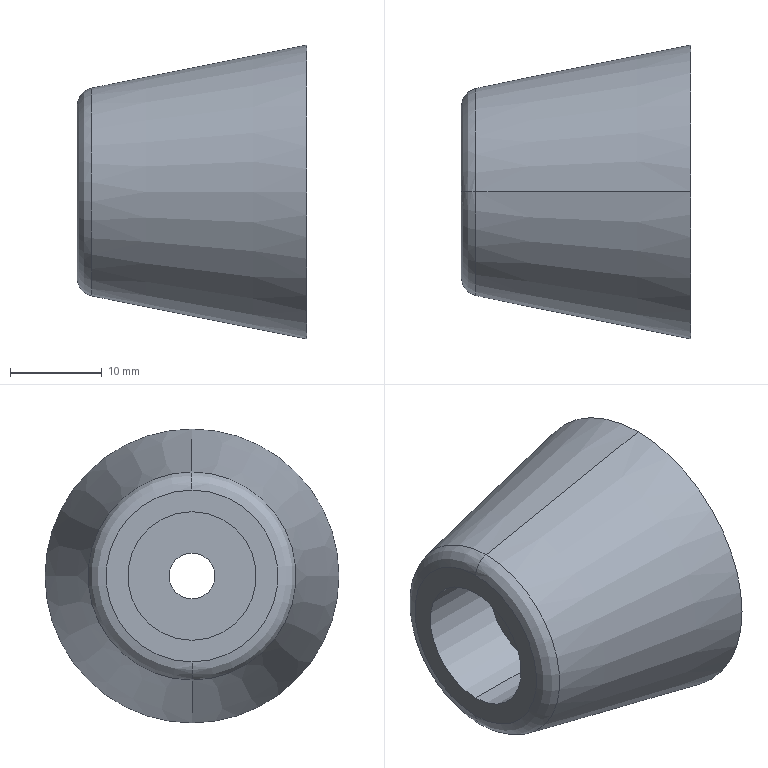Part | STEP file | NHY11-32 | 1 solid | 11 faces | box 25 x 32 x 32 mm | volume 12742 mm3 | cylinder 4 | plane 3 | cone 2 | torus 2 | commonest cylinder face diameters 5 x2 14 x2
STEP:
#1=CARTESIAN_POINT('',(1.608,0.000000013,11.322));
#2=VERTEX_POINT('',#1);
#3=CARTESIAN_POINT('',(1.608,-0.000000013,-11.322));
#4=VERTEX_POINT('',#3);
#5=CARTESIAN_POINT('',(1.608,0.,0.));
#6=DIRECTION('',(1.,0.,0.));
#7=DIRECTION('',(0.,0.,-1.));
#8=AXIS2_PLACEMENT_3D('',#5,#6,#7);
#9=CIRCLE('',#8,11.322);
#10=EDGE_CURVE('',#2,#4,#9,.T.);
#11=ORIENTED_EDGE('',*,*,#10,.T.);
#12=CARTESIAN_POINT('',(25.,-0.000000012,-16.));
#13=VERTEX_POINT('',#12);
#14=CARTESIAN_POINT('',(25.,-0.000000012,-16.));
#15=DIRECTION('',(0.9806,0.,-0.1961));
#16=VECTOR('',#15,1000.);
#17=LINE('',#14,#16);
#18=EDGE_CURVE('',#4,#13,#17,.T.);
#19=ORIENTED_EDGE('',*,*,#18,.T.);
#20=CARTESIAN_POINT('',(25.,0.000000012,16.));
#21=VERTEX_POINT('',#20);
#22=CARTESIAN_POINT('',(25.,0.,0.));
#23=DIRECTION('',(1.,0.,0.));
#24=DIRECTION('',(0.,0.,1.));
#25=AXIS2_PLACEMENT_3D('',#22,#23,#24);
#26=CIRCLE('',#25,16.);
#27=EDGE_CURVE('',#21,#13,#26,.T.);
#28=ORIENTED_EDGE('',*,*,#27,.F.);
#29=CARTESIAN_POINT('',(25.,0.000000012,16.));
#30=DIRECTION('',(0.9806,0.,0.1961));
#31=VECTOR('',#30,1000.);
#32=LINE('',#29,#31);
#33=EDGE_CURVE('',#2,#21,#32,.T.);
#34=ORIENTED_EDGE('',*,*,#33,.F.);
#35=EDGE_LOOP('',(#11,#19,#28,#34));
#36=FACE_OUTER_BOUND('',#35,.T.);
#37=CARTESIAN_POINT('',(25.,0.,0.));
#38=DIRECTION('',(1.,0.,0.));
#39=DIRECTION('',(0.,0.000000001,1.));
#40=AXIS2_PLACEMENT_3D('',#37,#38,#39);
#41=CONICAL_SURFACE('',#40,16.,0.1974);
#42=ADVANCED_FACE('',(#36),#41,.T.);
#43=CARTESIAN_POINT('',(9.,0.,-2.5));
#44=VERTEX_POINT('',#43);
#45=CARTESIAN_POINT('',(9.,-0.000000355,2.5));
#46=VERTEX_POINT('',#45);
#47=CARTESIAN_POINT('',(9.,0.,0.));
#48=DIRECTION('',(1.,0.,0.));
#49=DIRECTION('',(0.,-0.000000142,1.));
#50=AXIS2_PLACEMENT_3D('',#47,#48,#49);
#51=CIRCLE('',#50,2.5);
#52=EDGE_CURVE('',#44,#46,#51,.T.);
#53=ORIENTED_EDGE('',*,*,#52,.F.);
#54=CARTESIAN_POINT('',(25.,0.,-2.5));
#55=VERTEX_POINT('',#54);
#56=CARTESIAN_POINT('',(25.,0.,-2.5));
#57=DIRECTION('',(1.,0.,0.));
#58=VECTOR('',#57,1000.);
#59=LINE('',#56,#58);
#60=EDGE_CURVE('',#44,#55,#59,.T.);
#61=ORIENTED_EDGE('',*,*,#60,.T.);
#62=CARTESIAN_POINT('',(25.,0.,2.5));
#63=VERTEX_POINT('',#62);
#64=CARTESIAN_POINT('',(25.,0.,0.));
#65=DIRECTION('',(1.,0.,0.));
#66=DIRECTION('',(0.,0.,-1.));
#67=AXIS2_PLACEMENT_3D('',#64,#65,#66);
#68=CIRCLE('',#67,2.5);
#69=EDGE_CURVE('',#55,#63,#68,.T.);
#70=ORIENTED_EDGE('',*,*,#69,.T.);
#71=CARTESIAN_POINT('',(25.,0.,2.5));
#72=DIRECTION('',(1.,0.,0.));
#73=VECTOR('',#72,1000.);
#74=LINE('',#71,#73);
#75=EDGE_CURVE('',#46,#63,#74,.T.);
#76=ORIENTED_EDGE('',*,*,#75,.F.);
#77=EDGE_LOOP('',(#53,#61,#70,#76));
#78=FACE_OUTER_BOUND('',#77,.T.);
#79=CARTESIAN_POINT('',(25.,0.,0.));
#80=DIRECTION('',(1.,0.,0.));
#81=DIRECTION('',(0.,0.,1.));
#82=AXIS2_PLACEMENT_3D('',#79,#80,#81);
#83=CYLINDRICAL_SURFACE('',#82,2.5);
#84=ADVANCED_FACE('',(#78),#83,.F.);
#85=CARTESIAN_POINT('',(0.,0.,-7.));
#86=VERTEX_POINT('',#85);
#87=CARTESIAN_POINT('',(0.,0.,7.));
#88=VERTEX_POINT('',#87);
#89=CARTESIAN_POINT('',(0.,0.,0.));
#90=DIRECTION('',(1.,0.,0.));
#91=DIRECTION('',(0.,0.,1.));
#92=AXIS2_PLACEMENT_3D('',#89,#90,#91);
#93=CIRCLE('',#92,7.);
#94=EDGE_CURVE('',#86,#88,#93,.T.);
#95=ORIENTED_EDGE('',*,*,#94,.F.);
#96=CARTESIAN_POINT('',(9.,0.,-7.));
#97=VERTEX_POINT('',#96);
#98=CARTESIAN_POINT('',(25.,0.,-7.));
#99=DIRECTION('',(1.,0.,0.));
#100=VECTOR('',#99,1000.);
#101=LINE('',#98,#100);
#102=EDGE_CURVE('',#86,#97,#101,.T.);
#103=ORIENTED_EDGE('',*,*,#102,.T.);
#104=CARTESIAN_POINT('',(9.,0.,7.));
#105=VERTEX_POINT('',#104);
#106=CARTESIAN_POINT('',(9.,0.,0.));
#107=DIRECTION('',(1.,0.,0.));
#108=DIRECTION('',(0.,0.,-1.));
#109=AXIS2_PLACEMENT_3D('',#106,#107,#108);
#110=CIRCLE('',#109,7.);
#111=EDGE_CURVE('',#97,#105,#110,.T.);
#112=ORIENTED_EDGE('',*,*,#111,.T.);
#113=CARTESIAN_POINT('',(25.,0.,7.));
#114=DIRECTION('',(1.,0.,0.));
#115=VECTOR('',#114,1000.);
#116=LINE('',#113,#115);
#117=EDGE_CURVE('',#88,#105,#116,.T.);
#118=ORIENTED_EDGE('',*,*,#117,.F.);
#119=EDGE_LOOP('',(#95,#103,#112,#118));
#120=FACE_OUTER_BOUND('',#119,.T.);
#121=CARTESIAN_POINT('',(25.,0.,0.));
#122=DIRECTION('',(1.,0.,0.));
#123=DIRECTION('',(0.,0.,1.));
#124=AXIS2_PLACEMENT_3D('',#121,#122,#123);
#125=CYLINDRICAL_SURFACE('',#124,7.);
#126=ADVANCED_FACE('',(#120),#125,.F.);
#127=CARTESIAN_POINT('',(0.,0.000000012,9.36));
#128=VERTEX_POINT('',#127);
#129=CARTESIAN_POINT('',(0.,-0.000000012,-9.36));
#130=VERTEX_POINT('',#129);
#131=CARTESIAN_POINT('',(0.,0.,0.));
#132=DIRECTION('',(1.,0.,0.));
#133=DIRECTION('',(0.,0.,-1.));
#134=AXIS2_PLACEMENT_3D('',#131,#132,#133);
#135=CIRCLE('',#134,9.36);
#136=EDGE_CURVE('',#128,#130,#135,.T.);
#137=ORIENTED_EDGE('',*,*,#136,.T.);
#138=CARTESIAN_POINT('',(2.,-0.000000011,-9.36));
#139=DIRECTION('',(0.,-1.,0.000000001));
#140=DIRECTION('',(0.,-0.000000001,-1.));
#141=AXIS2_PLACEMENT_3D('',#138,#139,#140);
#142=CIRCLE('',#141,2.);
#143=EDGE_CURVE('',#130,#4,#142,.T.);
#144=ORIENTED_EDGE('',*,*,#143,.T.);
#145=ORIENTED_EDGE('',*,*,#10,.F.);
#146=CARTESIAN_POINT('',(2.,0.000000011,9.36));
#147=DIRECTION('',(0.,1.,-0.000000001));
#148=DIRECTION('',(0.,0.000000001,1.));
#149=AXIS2_PLACEMENT_3D('',#146,#147,#148);
#150=CIRCLE('',#149,2.);
#151=EDGE_CURVE('',#128,#2,#150,.T.);
#152=ORIENTED_EDGE('',*,*,#151,.F.);
#153=EDGE_LOOP('',(#137,#144,#145,#152));
#154=FACE_OUTER_BOUND('',#153,.T.);
#155=CARTESIAN_POINT('',(2.,0.,0.));
#156=DIRECTION('',(1.,0.,0.));
#157=DIRECTION('',(0.,0.000000001,1.));
#158=AXIS2_PLACEMENT_3D('',#155,#156,#157);
#159=TOROIDAL_SURFACE('',#158,9.36,2.);
#160=ADVANCED_FACE('',(#154),#159,.T.);
#161=ORIENTED_EDGE('',*,*,#136,.F.);
#162=CARTESIAN_POINT('',(0.,0.,0.));
#163=DIRECTION('',(1.,0.,0.));
#164=DIRECTION('',(0.,0.,-1.));
#165=AXIS2_PLACEMENT_3D('',#162,#163,#164);
#166=CIRCLE('',#165,9.36);
#167=EDGE_CURVE('',#130,#128,#166,.T.);
#168=ORIENTED_EDGE('',*,*,#167,.F.);
#169=EDGE_LOOP('',(#161,#168));
#170=FACE_OUTER_BOUND('',#169,.T.);
#171=CARTESIAN_POINT('',(0.,0.,0.));
#172=DIRECTION('',(1.,0.,0.));
#173=DIRECTION('',(0.,0.,1.));
#174=AXIS2_PLACEMENT_3D('',#171,#172,#173);
#175=CIRCLE('',#174,7.);
#176=EDGE_CURVE('',#88,#86,#175,.T.);
#177=ORIENTED_EDGE('',*,*,#176,.T.);
#178=ORIENTED_EDGE('',*,*,#94,.T.);
#179=EDGE_LOOP('',(#177,#178));
#180=FACE_BOUND('',#179,.T.);
#181=CARTESIAN_POINT('',(0.,-9.616,-9.36));
#182=DIRECTION('',(-1.,0.,0.));
#183=DIRECTION('',(0.,0.,1.));
#184=AXIS2_PLACEMENT_3D('',#181,#182,#183);
#185=PLANE('',#184);
#186=ADVANCED_FACE('',(#170,#180),#185,.T.);
#187=CARTESIAN_POINT('',(9.,0.,0.));
#188=DIRECTION('',(1.,0.,0.));
#189=DIRECTION('',(0.,0.,-1.));
#190=AXIS2_PLACEMENT_3D('',#187,#188,#189);
#191=CIRCLE('',#190,7.);
#192=EDGE_CURVE('',#105,#97,#191,.T.);
#193=ORIENTED_EDGE('',*,*,#192,.F.);
#194=ORIENTED_EDGE('',*,*,#111,.F.);
#195=EDGE_LOOP('',(#193,#194));
#196=FACE_OUTER_BOUND('',#195,.T.);
#197=CARTESIAN_POINT('',(9.,0.,0.));
#198=DIRECTION('',(1.,0.,0.));
#199=DIRECTION('',(0.,-0.000000142,1.));
#200=AXIS2_PLACEMENT_3D('',#197,#198,#199);
#201=CIRCLE('',#200,2.5);
#202=EDGE_CURVE('',#46,#44,#201,.T.);
#203=ORIENTED_EDGE('',*,*,#202,.T.);
#204=ORIENTED_EDGE('',*,*,#52,.T.);
#205=EDGE_LOOP('',(#203,#204));
#206=FACE_BOUND('',#205,.T.);
#207=CARTESIAN_POINT('',(9.,-7.191,-7.));
#208=DIRECTION('',(-1.,0.,0.));
#209=DIRECTION('',(0.,0.,1.));
#210=AXIS2_PLACEMENT_3D('',#207,#208,#209);
#211=PLANE('',#210);
#212=ADVANCED_FACE('',(#196,#206),#211,.T.);
#213=ORIENTED_EDGE('',*,*,#27,.T.);
#214=CARTESIAN_POINT('',(25.,0.,0.));
#215=DIRECTION('',(1.,0.,0.));
#216=DIRECTION('',(0.,0.,1.));
#217=AXIS2_PLACEMENT_3D('',#214,#215,#216);
#218=CIRCLE('',#217,16.);
#219=EDGE_CURVE('',#13,#21,#218,.T.);
#220=ORIENTED_EDGE('',*,*,#219,.T.);
#221=EDGE_LOOP('',(#213,#220));
#222=FACE_OUTER_BOUND('',#221,.T.);
#223=CARTESIAN_POINT('',(25.,0.,0.));
#224=DIRECTION('',(1.,0.,0.));
#225=DIRECTION('',(0.,0.,-1.));
#226=AXIS2_PLACEMENT_3D('',#223,#224,#225);
#227=CIRCLE('',#226,2.5);
#228=EDGE_CURVE('',#63,#55,#227,.T.);
#229=ORIENTED_EDGE('',*,*,#228,.F.);
#230=ORIENTED_EDGE('',*,*,#69,.F.);
#231=EDGE_LOOP('',(#229,#230));
#232=FACE_BOUND('',#231,.T.);
#233=CARTESIAN_POINT('',(25.,-16.297,16.));
#234=DIRECTION('',(1.,0.,0.));
#235=DIRECTION('',(0.,0.,-1.));
#236=AXIS2_PLACEMENT_3D('',#233,#234,#235);
#237=PLANE('',#236);
#238=ADVANCED_FACE('',(#222,#232),#237,.T.);
#239=ORIENTED_EDGE('',*,*,#143,.F.);
#240=ORIENTED_EDGE('',*,*,#167,.T.);
#241=ORIENTED_EDGE('',*,*,#151,.T.);
#242=CARTESIAN_POINT('',(1.608,0.,0.));
#243=DIRECTION('',(1.,0.,0.));
#244=DIRECTION('',(0.,0.,-1.));
#245=AXIS2_PLACEMENT_3D('',#242,#243,#244);
#246=CIRCLE('',#245,11.322);
#247=EDGE_CURVE('',#4,#2,#246,.T.);
#248=ORIENTED_EDGE('',*,*,#247,.F.);
#249=EDGE_LOOP('',(#239,#240,#241,#248));
#250=FACE_OUTER_BOUND('',#249,.T.);
#251=CARTESIAN_POINT('',(2.,0.,0.));
#252=DIRECTION('',(1.,0.,0.));
#253=DIRECTION('',(0.,0.000000001,1.));
#254=AXIS2_PLACEMENT_3D('',#251,#252,#253);
#255=TOROIDAL_SURFACE('',#254,9.36,2.);
#256=ADVANCED_FACE('',(#250),#255,.T.);
#257=ORIENTED_EDGE('',*,*,#102,.F.);
#258=ORIENTED_EDGE('',*,*,#176,.F.);
#259=ORIENTED_EDGE('',*,*,#117,.T.);
#260=ORIENTED_EDGE('',*,*,#192,.T.);
#261=EDGE_LOOP('',(#257,#258,#259,#260));
#262=FACE_OUTER_BOUND('',#261,.T.);
#263=CARTESIAN_POINT('',(25.,0.,0.));
#264=DIRECTION('',(1.,0.,0.));
#265=DIRECTION('',(0.,0.,1.));
#266=AXIS2_PLACEMENT_3D('',#263,#264,#265);
#267=CYLINDRICAL_SURFACE('',#266,7.);
#268=ADVANCED_FACE('',(#262),#267,.F.);
#269=ORIENTED_EDGE('',*,*,#60,.F.);
#270=ORIENTED_EDGE('',*,*,#202,.F.);
#271=ORIENTED_EDGE('',*,*,#75,.T.);
#272=ORIENTED_EDGE('',*,*,#228,.T.);
#273=EDGE_LOOP('',(#269,#270,#271,#272));
#274=FACE_OUTER_BOUND('',#273,.T.);
#275=CARTESIAN_POINT('',(25.,0.,0.));
#276=DIRECTION('',(1.,0.,0.));
#277=DIRECTION('',(0.,0.,1.));
#278=AXIS2_PLACEMENT_3D('',#275,#276,#277);
#279=CYLINDRICAL_SURFACE('',#278,2.5);
#280=ADVANCED_FACE('',(#274),#279,.F.);
#281=ORIENTED_EDGE('',*,*,#18,.F.);
#282=ORIENTED_EDGE('',*,*,#247,.T.);
#283=ORIENTED_EDGE('',*,*,#33,.T.);
#284=ORIENTED_EDGE('',*,*,#219,.F.);
#285=EDGE_LOOP('',(#281,#282,#283,#284));
#286=FACE_OUTER_BOUND('',#285,.T.);
#287=CARTESIAN_POINT('',(25.,0.,0.));
#288=DIRECTION('',(1.,0.,0.));
#289=DIRECTION('',(0.,0.000000001,1.));
#290=AXIS2_PLACEMENT_3D('',#287,#288,#289);
#291=CONICAL_SURFACE('',#290,16.,0.1974);
#292=ADVANCED_FACE('',(#286),#291,.T.);
#293=CLOSED_SHELL('',(#42,#84,#126,#160,#186,#212,#238,#256,#268,#280,#292));
#294=MANIFOLD_SOLID_BREP('',#293);
#295=CARTESIAN_POINT('',(0.,0.,0.));
#296=DIRECTION('',(0.,0.,1.));
#297=DIRECTION('',(1.,0.,0.));
#298=AXIS2_PLACEMENT_3D('',#295,#296,#297);
#299=(LENGTH_UNIT()NAMED_UNIT(*)SI_UNIT(.MILLI.,.METRE.));
#300=UNCERTAINTY_MEASURE_WITH_UNIT(LENGTH_MEASURE(0.00001),#299,'','');
#301=(NAMED_UNIT(*)PLANE_ANGLE_UNIT()SI_UNIT($,.RADIAN.));
#302=(NAMED_UNIT(*)SI_UNIT($,.STERADIAN.)SOLID_ANGLE_UNIT());
#303=(GEOMETRIC_REPRESENTATION_CONTEXT(3)GLOBAL_UNCERTAINTY_ASSIGNED_CONTEXT((#300))GLOBAL_UNIT_ASSIGNED_CONTEXT((#299,#301,#302))REPRESENTATION_CONTEXT('',''));
#304=ADVANCED_BREP_SHAPE_REPRESENTATION('',(#294,#298),#303);